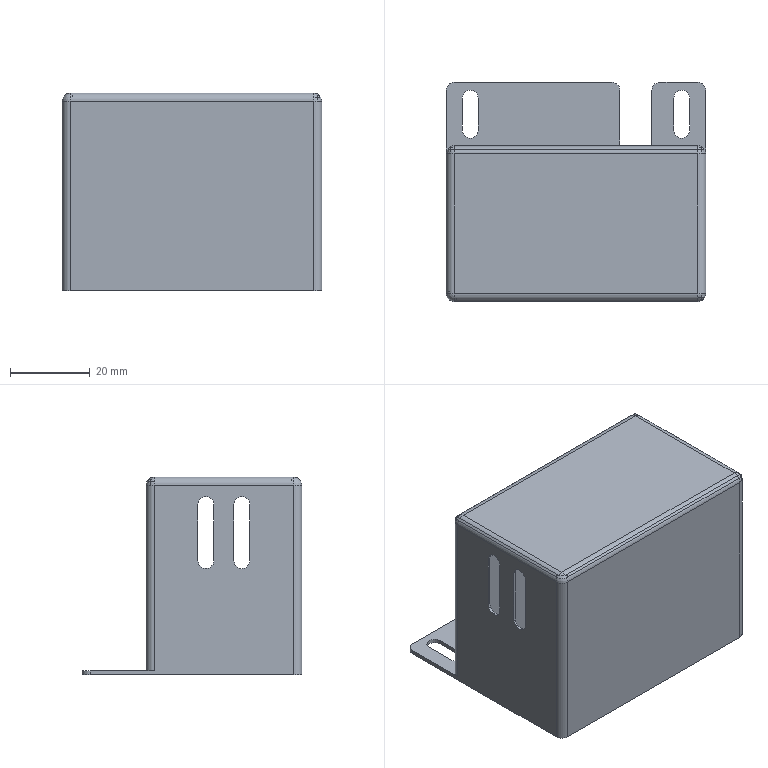Part | NX | features BREP 1 | 1 solid | 75 faces | box 65 x 55 x 49.5 mm | volume 6544 mm3 | cylinder 38 | plane 29 | sphere 7 | torus 1 | commonest cylinder face diameters 4 x29 1 x7 8 x2